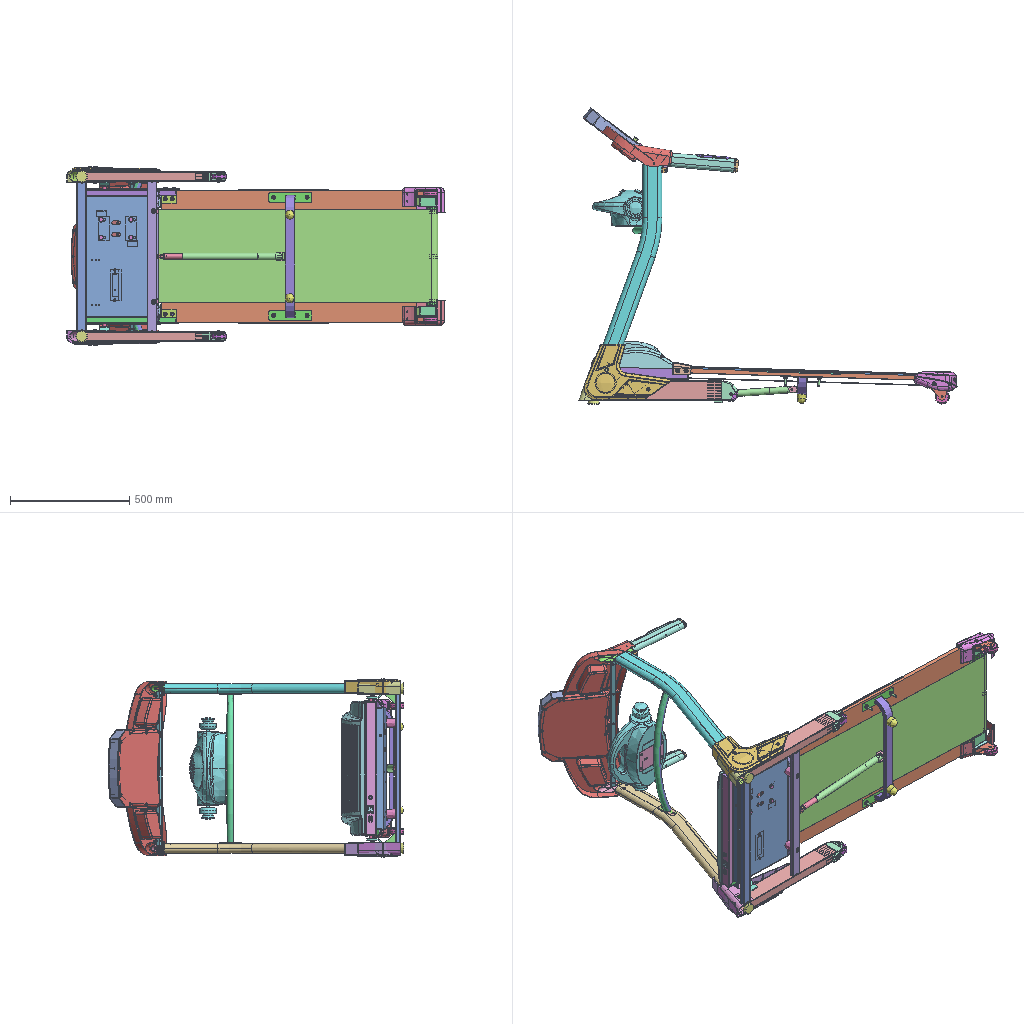Assembly | STEP file | 108 different items | 216 placed | box 1585 x 1241 x 747 mm
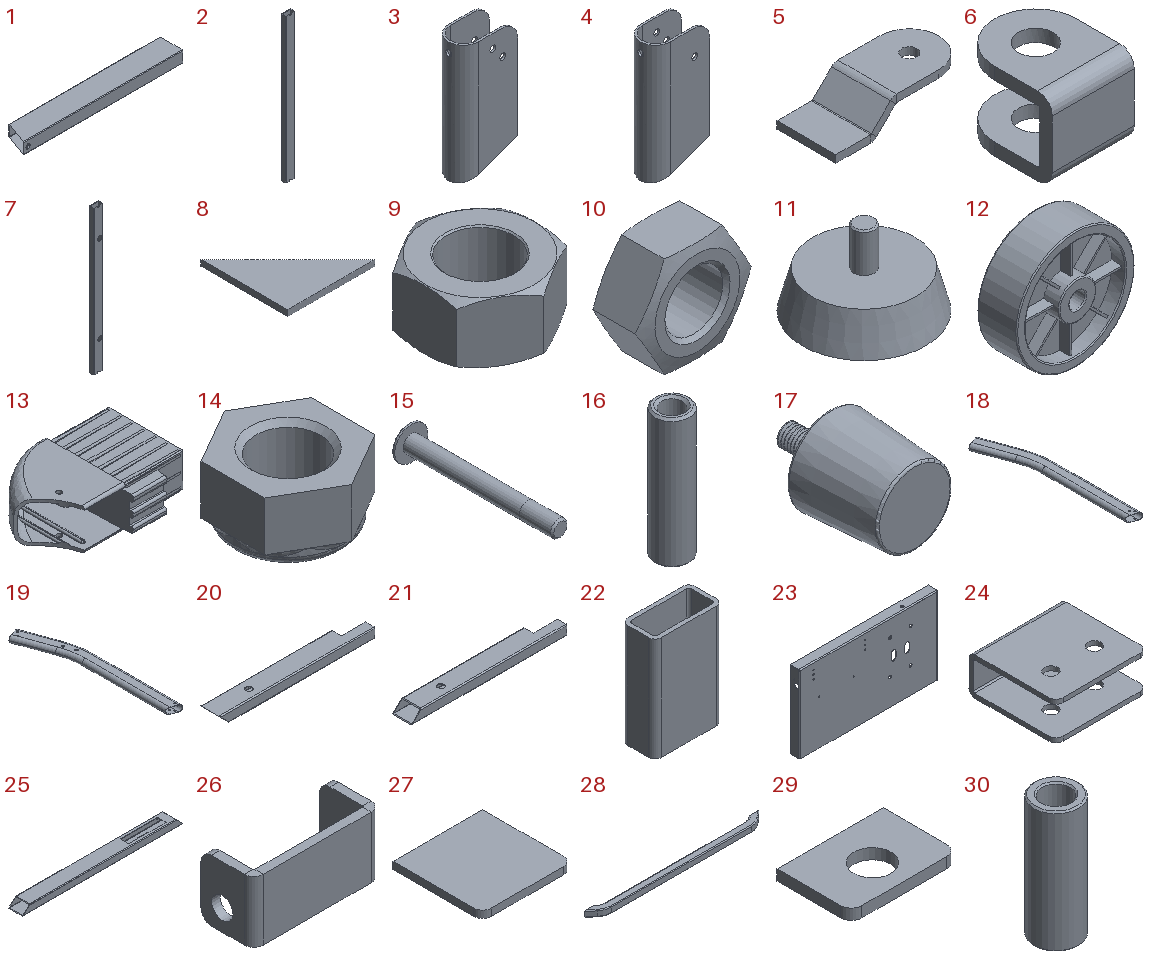Parts list (item | name | quantity | parent item | size | volume):
1 | 5090101 | x2 | in 5090100 | 550 x 80 x 40 mm | 185626 mm3
2 | 5090102 | x1 | in 5090100 | 40 x 20 x 624 mm | 103774 mm3
3 | 5090103L | x1 | in 5090100 | 83 x 46 x 184 mm | 94323 mm3
4 | 5090103R | x1 | in 5090100 | 83 x 46 x 184 mm | 94323 mm3
5 | 5090104 | x2 | in 5090100 | 90 x 40 x 20 mm | 17915 mm3
6 | PN_0010_default | x3 | in 5090100, 5090200L, 5090200R | 20 x 24 x 19 mm | 2959 mm3
7 | 5090107 | x1 | in 5090100 | 40 x 20 x 630 mm | 102888 mm3
8 | 5090108 | x2 | in 5090100 | 45 x 45 x 3 mm | 3037 mm3
9 | N1101210 | x4 | in 5090100, 5091300 | 16.454 x 19 x 9 mm | 1389 mm3
10 | N108078 | x10 | in 5090100, 5090200L, 5090200R, 5091200 | 16 x 7 x 13.856 mm | 779.97 mm3
11 | 5090101W | x2 | in 5090100Z | 47.789 x 47.789 x 30.5 mm | 24412 mm3
12 | PN_0007_default | x2 | in 5090100Z | 60 x 22 x 60 mm | 32782 mm3
13 | PN_0011_default | x2 | in 5090100Z | 130 x 91 x 40 mm | 95148 mm3
14 | PN_0002 | x2 | in 5090100Z | 8.5 x 9.815 x 5.1 mm | 204.852 mm3
15 | SD10545 | x2 | in 5090100Z | 10 x 47.433 x 10 mm | 991.806 mm3
16 | 5090905 | x2 | in 5090100Z | 8.2 x 8.2 x 31 mm | 968.239 mm3
17 | 5090104W | x2 | in 5090100Z | 39.871 x 60 x 39.871 mm | 45524 mm3
18 | 5090201L | x1 | in 5090200L | 181.681 x 917.444 x 40 mm | 273623 mm3
19 | 5090201R | x1 | in 5090200R | 181.681 x 917.444 x 40 mm | 273224 mm3
20 | 5090501L | x1 | in 5090500 | 400 x 50 x 25 mm | 74106 mm3
21 | 5090501R | x1 | in 5090500 | 400 x 50 x 25 mm | 74487 mm3
22 | 5090502 | x2 | in 5090500 | 26 x 13 x 40 mm | 4140 mm3
23 | 5090503 | x1 | in 5090500 | 508 x 35 x 285 mm | 354091 mm3
24 | 5090504 | x4 | in 5090500, 5091400L, 5091400R | 63 x 60 x 26 mm | 24845 mm3
25 | 5090505 | x1 | in 5090500 | 558 x 50 x 25 mm | 105328 mm3
26 | 5090506 | x1 | in 5090500 | 60 x 25 x 29 mm | 10869 mm3
27 | 5090507 | x2 | in 5090500 | 25 x 25 x 2 mm | 1245 mm3
28 | 5090508 | x1 | in 5090500 | 550.086 x 30 x 20 mm | 56532 mm3
29 | 5090509 | x1 | in 5090500 | 50 x 35 x 5 mm | 7494 mm3
30 | 5090510 | x2 | in 5090500 | 15.8 x 15.8 x 43 mm | 5033 mm3
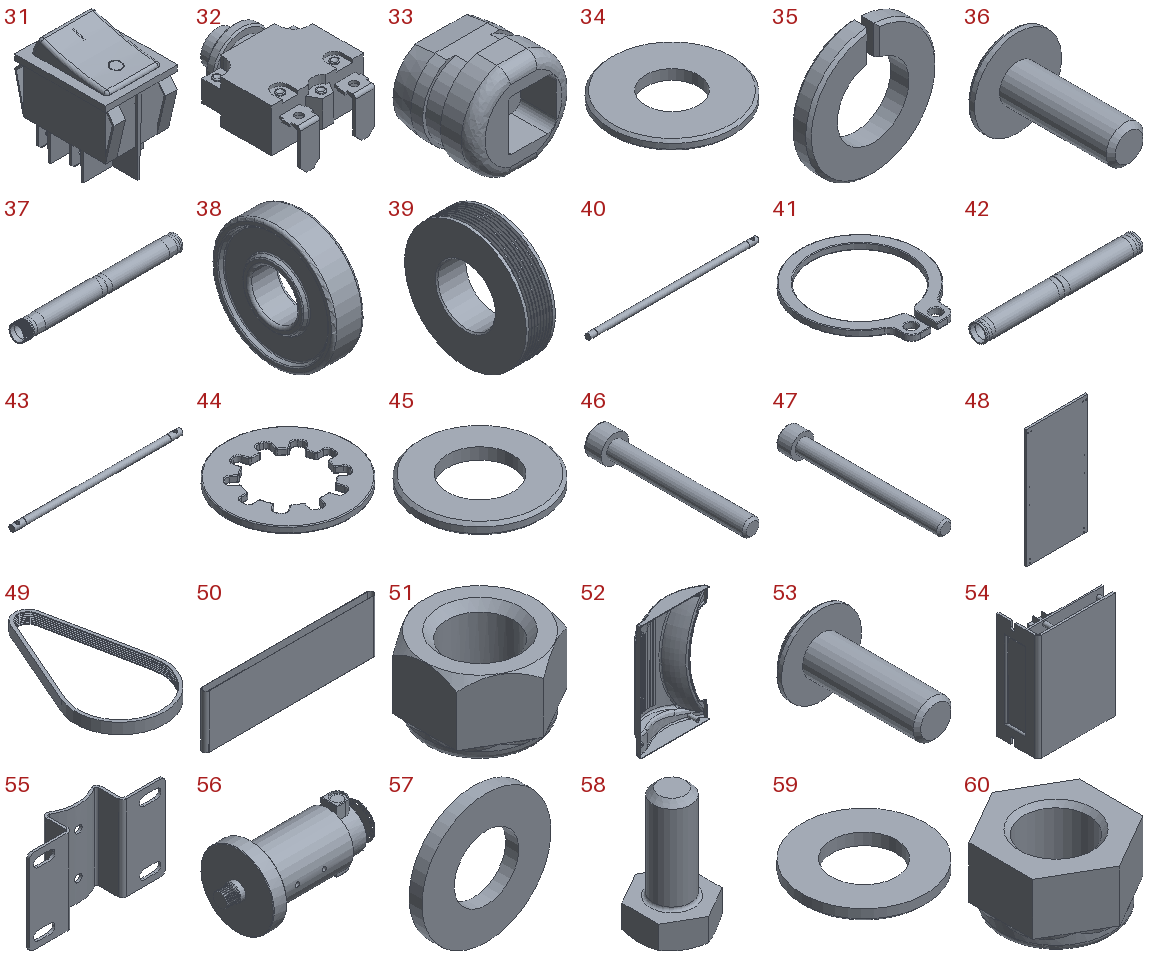31 | EP002 | x1 | in 5090500Z | 25 x 34.5 x 34.784 mm | 14567 mm3
32 | EC002 | x1 | in 5090500Z | 29.3 x 39.3 x 19.65 mm | 10331 mm3
33 | PN_0006_default | x1 | in 5090500Z | 17 x 14 x 16 mm | 1519 mm3
34 | PN_0009 | x3 | in 5090500Z | 9.8 x 9.8 x 0.8 mm | 48.045 mm3
35 | W204009 | x3 | in 5090500Z | 9.2 x 1.3 x 9.193 mm | 57.255 mm3
36 | SD10412 | x3 | in 5090500Z | 9.4 x 14.503 x 9.4 mm | 245.335 mm3
37 | 5090701 | x1 | in 5090700Z | 460 x 46 x 46 mm | 209317 mm3
38 | PL6203ZZA_default | x4 | in 5090700Z, 5090800Z | 11 x 44 x 44 mm | 11669 mm3
39 | PN_0004_default | x1 | in 5090700Z | 23 x 96 x 96 mm | 121730 mm3
40 | 5090702 | x1 | in 5090700Z | 513 x 17 x 17 mm | 116620 mm3
41 | PN_0013 | x4 | in 5090700Z, 5090800Z | 19 x 21.5 x 1 mm | 101.865 mm3
42 | 5090801 | x1 | in 5090800Z | 410 x 46 x 46 mm | 188992 mm3
43 | 5090802 | x1 | in 5090800Z | 480 x 17 x 17 mm | 107509 mm3
44 | PN_0005 | x3 | in 5090500Z | 15 x 15 x 0.8 mm | 82.689 mm3
45 | PN_0008 | x15 | in 5090500Z | 17 x 17 x 1.6 mm | 252.969 mm3
46 | SA10865 | x1 | in 5090500Z | 13 x 73 x 13 mm | 4160 mm3
47 | SA10880 | x2 | in 5090500Z | 13 x 88 x 13 mm | 4914 mm3
48 | DECK509 | x1 | in 5090500Z | 554 x 18 x 1070 mm | 10652247 mm3
49 | DE170J509 | x1 | in 5090500Z | 99 x 178.5 x 12 mm | 14354 mm3
50 | RUBE509 | x1 | in 5090500Z | 1253 x 49.2 x 390 mm | 1595905 mm3
51 | PN_0001 | x2 | in 5090500Z | 10 x 11.547 x 7 mm | 381.046 mm3
52 | MOCV509 | x1 | in 5090500Z | 342.742 x 110.913 x 567 mm | 804281 mm3
53 | SD10515 | x2 | in 5090500Z | 10.5 x 17.955 x 10.5 mm | 436.429 mm3
54 | 509K1002 | x1 | in 5090500Z | 93.5 x 58.5 x 129.5 mm | 128937 mm3
55 | 5090601 | x1 | in 5090500Z | 160 x 33 x 100 mm | 61520 mm3
56 | MOTOR default | x1 | in 5090500Z | 260 x 138 x 138 mm | 1629654 mm3
57 | 509~20.10.T2.0 | x4 | in 5090500Z | 20 x 2 x 20 mm | 471.239 mm3
58 | SI1025_M10 | x4 | in 5090500Z | 17 x 19.6 x 32 mm | 3678 mm3
59 | W110020_M10 | x4 | in 5090500Z | 21 x 21 x 2 mm | 494.539 mm3
60 | N210095 | x4 | in 5090500Z | 17 x 19.63 x 10.5 mm | 1722 mm3
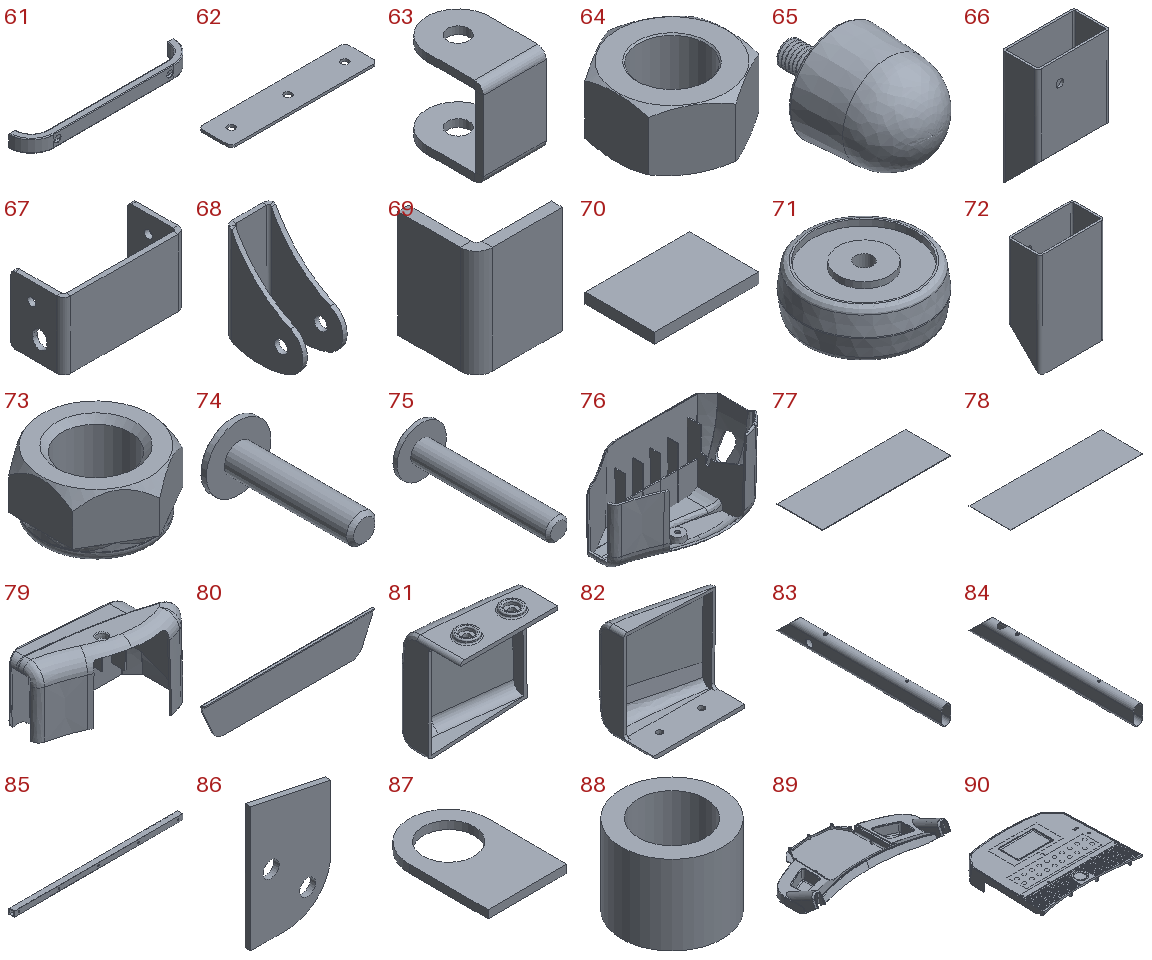61 | 5091301 | x1 | in 5091300 | 515 x 70 x 40 mm | 91933 mm3
62 | 5091302 | x2 | in 5091300 | 180 x 40 x 3 mm | 20963 mm3
63 | 5091303 | x1 | in 5091300 | 25 x 35 x 35 mm | 6553 mm3
64 | N1101215 | x1 | in 5091300 | 16.454 x 19 x 9 mm | 1389 mm3
65 | 5091301W | x2 | in 5091300Z | 39.871 x 60 x 39.871 mm | 39857 mm3
66 | 5091401L | x1 | in 5091400L | 50 x 25 x 80 mm | 14246 mm3
67 | 5091402 | x2 | in 5091400L, 5091400R | 76 x 33 x 42 mm | 16188 mm3
68 | 5091403 | x2 | in 5091400L, 5091400R | 30 x 53 x 70.522 mm | 17329 mm3
69 | 5091404 | x2 | in 5091400L, 5091400R | 24 x 22 x 30 mm | 3754 mm3
70 | 5091405 | x2 | in 5091400L, 5091400R | 30 x 20 x 3 mm | 1800 mm3
71 | Transport wheel | x2 | in 5091400LZ, 5091400RZ | 59.962 x 59.962 x 23 mm | 51034 mm3
72 | 5091401R | x1 | in 5091400R | 50 x 25 x 80 mm | 14246 mm3
73 | N208078 | x12 | in 5090500Z | 13.017 x 15.011 x 7.5 mm | 666.866 mm3
74 | PN_0012 | x6 | in 5090500Z | 18 x 39.451 x 18 mm | 2453 mm3
75 | PN_0003 | x4 | in 5090500Z | 18 x 54.451 x 18 mm | 3207 mm3
76 | END CAP R | x1 | in 5090500Z | 178.531 x 81.742 x 105 mm | 112295 mm3
77 | JZHM | x1 | in 5090500Z | 1060 x 370 x 5 mm | 1961000 mm3
78 | JZBM | x1 | in 5090500Z | 1170 x 370 x 1.5 mm | 649350 mm3
79 | END CAP L | x1 | in 5090500Z | 178.531 x 81.742 x 105 mm | 112297 mm3
80 | Plastic anti-slip plate | x2 | in 5090500Z | 380 x 9.3 x 80 mm | 74474 mm3
81 | HGL | x1 | in 5090500Z | 76.93 x 46.944 x 81.839 mm | 29643 mm3
82 | HGR | x1 | in 5090500Z | 76.93 x 46.944 x 81.839 mm | 29457 mm3
83 | 5091201L | x1 | in 5091200 | 25 x 430 x 50 mm | 72526 mm3
84 | 5091201R | x1 | in 5091200 | 25 x 430 x 50 mm | 72112 mm3
85 | 5091202 | x1 | in 5091200 | 645 x 20 x 20 mm | 70797 mm3
86 | 5091203 | x2 | in 5091200 | 45 x 3 x 70 mm | 8020 mm3
87 | PN_0014_default | x2 | in 5091200 | 20 x 30 x 2 mm | 848.625 mm3
88 | 5091205 | x2 | in 5091200 | 12.7 x 12.7 x 10 mm | 699.319 mm3
89 | 5091204W | x1 | in 5091200ZA | 729.86 x 412.544 x 132.193 mm | 994428 mm3
90 | 5091205W | x1 | in 5091200ZA | 340.656 x 315.859 x 50.2 mm | 442857 mm3
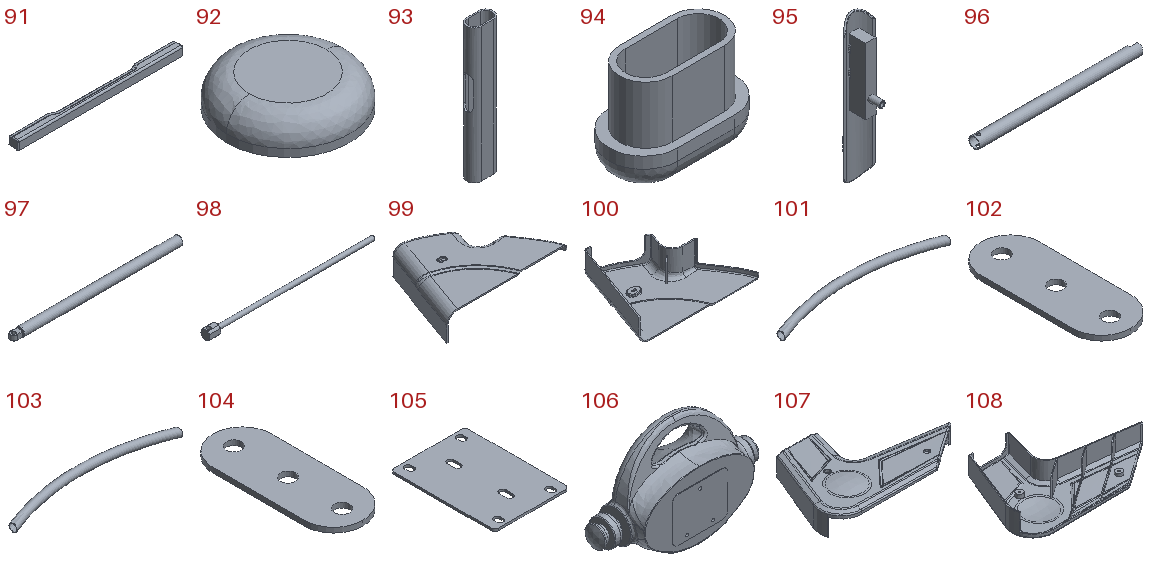91 | 5091206W | x1 | in 5091200ZA | 329.891 x 19 x 17 mm | 29146 mm3
92 | 5091207W | x1 | in 5091200ZA | 32 x 32 x 8 mm | 5722 mm3
93 | 5091202W | x2 | in 5091200Z | 56 x 31 x 280 mm | 111520 mm3
94 | 5091201W | x2 | in 5091200Z | 55 x 30 x 40 mm | 14553 mm3
95 | 5091203W | x2 | in 5091200Z | 31 x 32.516 x 144.3 mm | 20924 mm3
96 | GAS SHOCK A01W | x1 | in 509 | 420 x 28 x 28 mm | 51028 mm3
97 | GAS SHOCK A01X | x1 | in 509 | 419 x 22 x 22 mm | 110141 mm3
98 | GAS SHOCK A01S | x1 | in 509 | 398.5 x 20 x 20 mm | 38228 mm3
99 | LZHT-L1 | x1 | in 509 | 250 x 180.091 x 55 mm | 105552 mm3
100 | LZHT-R1 | x1 | in 509 | 250 x 180.091 x 55 mm | 106562 mm3
101 | 5091501 | x1 | in 5091500 | 620 x 92.341 x 28.6 mm | 81368 mm3
102 | 5091502 | x2 | in 5091500 | 35 x 90 x 3 mm | 8089 mm3
103 | 5091501M | x1 | in 5091500M | 620 x 92.341 x 28.6 mm | 81368 mm3
104 | 5091502M | x2 | in 5091500M | 35 x 90 x 3 mm | 8090 mm3
105 | 5091503M | x1 | in 5091500M | 100 x 140 x 3 mm | 39981 mm3
106 | 5091504W | x1 | in 5091500MA | 430 x 154.443 x 270 mm | 5728271 mm3
107 | BLZHT2-L | x1 | in 509 | 369.553 x 235 x 62.57 mm | 247383 mm3
108 | BLZHT2-R | x1 | in 509 | 369.553 x 235 x 62.57 mm | 247381 mm3
Placements (level | parent | child | x y z in mm | rotation matrix by rows):
1 | 509 | 5090100Z | 20.74 99.795 0.0 | 1 0 0 0 1 0 0 0 1
2 | 5090100Z | 5090100 | -0.0 -0.0 -0.0 | 1 0 0 0 1 0 0 0 1
3 | 5090100 | 5090101 | -0.0 -0.0 -0.0 | 1 0 0 0 1 0 0 0 1
3 | 5090100 | 5090101 | 0.0 -0.0 -670.0 | 1 0 0 0 1 0 0 0 1
3 | 5090100 | 5090102 | -535.0 -0.0 -335.0 | 1 0 0 0 1 0 0 0 1
3 | 5090100 | 5090103L | -526.578 -33.334 0.0 | 0.9397 0 0.342 -0.342 0 0.9397 0 -1 0
3 | 5090100 | 5090103R | -526.578 -33.334 -670.0 | 0.9397 0 0.342 -0.342 0 0.9397 0 -1 -0
3 | 5090100 | 5090104 | -440.0 121.5 -35.0 | 0 1 0 1 0 0 0 0 -1
3 | 5090100 | PN_0010_default | -220.0 10.0 -335.0 | 0 1 0 -1 0 0 0 0 1
3 | 5090100 | 5090104 | -440.0 121.5 -635.0 | 0 -1 0 1 0 0 0 0 1
3 | 5090100 | 5090107 | -240.0 -0.0 -335.0 | 1 0 0 0 1 0 0 0 1
3 | 5090100 | 5090108 | -535.0 28.721 -610.721 | 0 0 1 1 0 0 0 1 -0
3 | 5090100 | N1101210 | -233.0 11.0 -145.0 | 1 0 0 0 0 1 0 -1 0
3 | 5090100 | N1101210 | -233.0 20.0 -525.0 | 1 0 0 0 0 -1 0 1 0
3 | 5090100 | N108078 | -479.683 116.674 -26.5 | 0.7825 0 0.6226 0.6226 0 -0.7825 0 1 -0
3 | 5090100 | N108078 | -479.683 116.674 -643.5 | 0.7825 0 -0.6226 0.6226 0 0.7825 0 -1 -0
3 | 5090100 | 5090108 | -532.0 28.721 -59.279 | 0 0 -1 1 0 0 0 -1 -0
2 | 5090100Z | 5090101W | -535.0 -0.0 -0.0 | 1 0 0 0 0 1 0 -1 0
2 | 5090100Z | PN_0007_default | 40.0 25.0 -11.0 | 1 0 0 0 0 -1 0 1 -0
2 | 5090100Z | PN_0011_default | 70.0 80.0 20.0 | -1 0 0 0 1 0 0 0 -1
2 | 5090100Z | PN_0002 | 40.0 25.0 -23.8 | 1 0 0 0 1 0 0 0 1
2 | 5090100Z | SD10545 | 40.0 25.0 20.0 | 1 0 0 0 0 -1 0 1 0
2 | 5090100Z | 5090905 | 40.0 25.0 15.5 | 1 0 0 0 1 0 0 0 1
2 | 5090100Z | 5090101W | -535.0 -0.0 -670.0 | -1 0 0 0 0 1 0 1 0
2 | 5090100Z | PN_0007_default | 40.0 25.0 -659.0 | -1 0 0 0 0 -1 0 -1 0
2 | 5090100Z | SD10545 | 40.0 25.0 -690.0 | 1 0 0 0 0 1 0 -1 0
2 | 5090100Z | 5090905 | 40.0 25.0 -654.5 | 1 0 0 0 1 0 0 0 1
2 | 5090100Z | PN_0002 | 40.0 25.0 -646.2 | -1 0 0 0 1 0 0 0 -1
2 | 5090100Z | PN_0011_default | 70.0 80.0 -649.992 | -1 0 0 0 1 0 0 0 -1
2 | 5090100Z | 5090104W | -233.0 -8.863 -145.0 | -0.8372 0 -0.5469 0 -1 0 -0.5469 0 0.8372
2 | 5090100Z | 5090104W | -233.0 -8.863 -525.0 | -0.8372 0 0.5469 0 -1 0 0.5469 0 0.8372
1 | 509 | 5090200L | -333.426 643.809 0.0 | 0.9397 0.342 0 -0.342 0.9397 0 0 0 1
2 | 5090200L | 5090201L | -26.789 -424.56 -0.0 | 1 0 0 0 1 0 0 0 1
2 | 5090200L | PN_0010_default | -44.744 430.969 -0.0 | -0.342 0.9397 0 0.9397 0.342 0 0 0 -1
2 | 5090200L | N108078 | 13.211 -426.268 15.0 | 1 0 0 0 0 -1 0 1 0
2 | 5090200L | N108078 | -20.385 -421.442 -0.0 | 0 -1 0 -0.4254 0 -0.905 0.905 0 -0.4254
1 | 509 | 5090200R | -356.082 649.787 -670.0 | 0.9397 0.342 0 -0.342 0.9397 0 0 0 1
2 | 5090200R | 5090201R | -3.454 -422.429 -0.0 | 1 0 0 0 1 0 0 0 1
2 | 5090200R | PN_0010_default | -21.409 433.101 -0.0 | 0.342 0.9397 0 -0.9397 0.342 0 0 0 1
2 | 5090200R | N108078 | 36.546 -424.137 -15.0 | 1 0 0 0 0 -1 0 1 0
2 | 5090200R | N108078 | 2.636 -419.311 -0.0 | 0 -1 0 -0.9664 0 0.2572 -0.2572 0 -0.9664
1 | 509 | 5090500Z | -120.17 187.087 -67.5 | 0.9995 0.03073 0 -0.03073 0.9995 0 0 0 1
2 | 5090500Z | 5090500 | -0.0 -0.0 -0.0 | 1 0 0 0 1 0 0 0 1
3 | 5090500 | 5090501L | -0.0 -0.0 -0.0 | 1 0 0 0 1 0 0 0 1
3 | 5090500 | 5090501R | -0.0 0.0 -535.0 | 1 0 0 0 1 0 0 0 1
3 | 5090500 | 5090502 | -311.0 -21.5 -87.5 | 0 0 1 0 1 0 -1 0 0
3 | 5090500 | 5090502 | -181.0 -21.5 -214.5 | 0 0 -1 0 1 0 1 0 0
3 | 5090500 | 5090503 | -375.0 -30.0 -267.5 | 0 0 -1 0 1 0 1 0 -0
3 | 5090500 | 5090504 | -29.5 37.0 -546.5 | 1 0 0 0 0 1 0 -1 -0
3 | 5090500 | 5090504 | -29.5 37.0 11.5 | 1 0 0 0 0 -1 0 1 -0
3 | 5090500 | 5090505 | -387.5 25.0 -267.5 | 0 0 1 0 1 0 -1 0 -0
3 | 5090500 | 5090506 | -130.0 14.0 -507.0 | -1 0 0 0 1 0 0 0 -1
3 | 5090500 | 5090507 | 2.0 11.5 -0.0 | 0 0 -1 0 1 0 1 0 0
3 | 5090500 | 5090508 | -80.0 -20.0 -267.5 | 0 0 1 0 1 0 -1 0 -0
3 | 5090500 | 5090509 | -130.0 44.0 -17.5 | -1 0 0 0 -1 0 0 0 1
3 | 5090500 | 5090510 | -300.0 25.0 4.0 | 0.9768 -0.2143 0 0.2143 0.9768 0 0 0 1
3 | 5090500 | 5090510 | -300.0 25.0 -539.0 | 0.9768 -0.2143 0 0.2143 0.9768 0 0 0 1
3 | 5090500 | 5090507 | 2.0 11.5 -535.0 | 0 0 -1 0 1 0 1 0 0
2 | 5090500Z | EP002 | -400.0 24.95 -438.75 | 0 0 -1 1 0 0 0 -1 -0
2 | 5090500Z | EC002 | -342.72 18.1 -435.835 | 0 -1 0 0 0 -1 1 0 0
2 | 5090500Z | PN_0006_default | -405.5 24.764 -388.797 | 0 1 0 -1 0 0 0 0 1
2 | 5090500Z | PN_0009 | -255.0 -24.7 -451.5 | 1 0 0 0 0 -1 0 1 -0
2 | 5090500Z | PN_0009 | -254.0 -19.7 -406.5 | -0.9887 -0.15 0 0 0 -1 0.15 -0.9887 -0
2 | 5090500Z | PN_0009 | -255.0 -24.7 -323.5 | 1 0 0 0 0 -1 0 1 -0
2 | 5090500Z | W204009 | -254.0 -19.7 -406.5 | -0.9887 0 -0.15 0 1 0 0.15 0 -0.9887
2 | 5090500Z | W204009 | -255.0 -24.7 -451.5 | 1 0 0 0 1 0 0 0 1
2 | 5090500Z | W204009 | -255.0 -24.7 -323.5 | 1 0 0 0 1 0 0 0 1
2 | 5090500Z | SD10412 | -255.0 -23.4 -323.5 | 0.6736 0 -0.7391 0 1 0 0.7391 0 0.6736
2 | 5090500Z | SD10412 | -254.0 -18.4 -406.5 | 0.923 0 0.3849 0 1 0 -0.3849 0 0.923
2 | 5090500Z | SD10412 | -255.0 -23.4 -451.5 | -0.7187 0 0.6953 0 1 0 -0.6953 0 -0.7187
2 | 5090500Z | 5090700Z | -130.0 29.0 -266.7 | 0 0 1 0 1 0 -1 0 -0
3 | 5090700Z | 5090701 | 0.0 -0.0 0.0 | 1 0 0 0 1 0 0 0 1
3 | 5090700Z | PL6203ZZA_default | -241.0 8.5 -0.0 | 1 0 0 0 1 0 0 0 1
3 | 5090700Z | PL6203ZZA_default | 208.0 8.5 -0.0 | 1 0 0 0 1 0 0 0 1
3 | 5090700Z | PN_0004_default | -218.0 -0.0 0.0 | -1 0 0 0 0.5305 0.8477 0 0.8477 -0.5305
3 | 5090700Z | 5090702 | -7.7 -0.0 0.0 | 1 0 0 0 1 0 0 0 1
3 | 5090700Z | PN_0013 | 220.1 -0.0 0.0 | 0 0 -1 0 1 0 1 0 0
3 | 5090700Z | PN_0013 | -242.1 -0.0 0.0 | 0 0 1 0 1 0 -1 0 0
2 | 5090500Z | 5090800Z | 1074 30.0 -267.0 | 0 0 -1 0 -1 0 -1 0 0
3 | 5090800Z | 5090801 | -0.0 0.0 0.0 | 1 0 0 0 1 0 0 0 1
3 | 5090800Z | 5090802 | -0.0 0.0 0.0 | 1 0 0 0 1 0 0 0 1
3 | 5090800Z | PL6203ZZA_default | -205.0 8.5 -0.0 | 1 0 0 0 1 0 0 0 1
3 | 5090800Z | PL6203ZZA_default | 194.0 8.5 -0.0 | 1 0 0 0 1 0 0 0 1
3 | 5090800Z | PN_0013 | 205.9 0.0 0.0 | 0 0 -1 0 1 0 1 0 0
3 | 5090800Z | PN_0013 | -206.1 0.0 0.0 | 0 0 1 0 1 0 -1 0 -0
2 | 5090500Z | PN_0005 | -160.8 29.0 -502.5 | 0 0 1 -0.6832 -0.7302 0 0.7302 -0.6832 -0
2 | 5090500Z | PN_0005 | 1095.25 30.0 -42.0 | 0 0 1 0.4022 -0.9156 0 0.9156 0.4022 -0
2 | 5090500Z | PN_0005 | 1095.25 30.0 -492.0 | 0 0 1 1 0.003456 0 -0.003456 1 -0
2 | 5090500Z | PN_0008 | -162.4 29.0 -502.5 | 0 0 1 0 1 0 -1 0 0
2 | 5090500Z | PN_0008 | 1097.65 30.0 -492.0 | 0 0 -1 0.4285 -0.9035 0 -0.9035 -0.4285 0
2 | 5090500Z | SA10865 | -162.4 29.0 -502.5 | 0 -1 0 0.4079 0 -0.913 0.913 0 0.4079
2 | 5090500Z | SA10880 | 1097.65 30.0 -42.0 | 0 1 0 -0.354 0 0.9352 0.9352 0 0.354
2 | 5090500Z | SA10880 | 1097.65 30.0 -492.0 | 0 1 0 0.4455 0 0.8953 0.8953 0 -0.4455
2 | 5090500Z | DECK509 | 1010.25 27.0 -267.5 | 0 0 1 0 1 0 -1 0 -0
2 | 5090500Z | DE170J509 | 164.593 508.146 -37.7 | 0.04897 -0.9988 0 0.9988 0.04897 0 0 0 1
2 | 5090500Z | RUBE509 | 1118.5 30.037 -267.5 | 1 -0.000831 0 0.000831 1 0 0 0 1
2 | 5090500Z | PN_0001 | -126.878 5.5 -32.5 | 1 0 0 0 0 1 0 -1 0
2 | 5090500Z | PN_0001 | -126.878 5.5 -502.5 | 1 0 0 0 0 1 0 -1 -0
2 | 5090500Z | MOCV509 | -404.004 41.0 -267.496 | 1 0 0 0 1 0 0 0 1
2 | 5090500Z | SD10515 | 1097.25 35.0 -510.0 | 0 1 0 -0.4667 0 0.8844 0.8844 0 0.4667
2 | 5090500Z | SD10515 | 1097.25 35.0 -25.0 | 0 1 0 0.957 0 -0.29 -0.29 0 -0.957
2 | 5090500Z | 509K1002 | -226.5 -25.5 -453.507 | 0 -1 0 1 0 0 0 0 1
2 | 5090500Z | 5090601 | -243.269 -23.0 -151.0 | 1 0 0 0 1 0 0 0 1
2 | 5090500Z | MOTOR default | -243.269 46.7 -27.5 | 0 0 1 0 1 0 -1 0 -0
2 | 5090500Z | 509~20.10.T2.0 | -186.5 -28.0 -113.5 | 1 0 0 0 1 0 0 0 1
2 | 5090500Z | SI1025_M10 | -186.5 -37.0 -113.5 | 0.9832 -0.1826 0 0 0 1 -0.1826 -0.9832 0
2 | 5090500Z | W110020_M10 | -186.5 -21.0 -113.5 | 1 0 0 0 0 -1 0 1 -0
2 | 5090500Z | N210095 | -186.5 -13.0 -113.5 | 1 0 0 0 0 -1 0 1 -0
2 | 5090500Z | 509~20.10.T2.0 | -311.5 -28.0 -113.5 | 1 0 0 0 1 0 0 0 1
2 | 5090500Z | 509~20.10.T2.0 | -186.5 -28.0 -188.5 | 1 0 0 0 1 0 0 0 1
2 | 5090500Z | 509~20.10.T2.0 | -311.5 -28.0 -188.5 | 1 0 0 0 1 0 0 0 1
2 | 5090500Z | W110020_M10 | -311.5 -21.0 -113.5 | 1 0 0 0 0 -1 0 1 -0
2 | 5090500Z | W110020_M10 | -186.5 -21.0 -188.5 | 1 0 0 0 0 -1 0 1 -0
2 | 5090500Z | W110020_M10 | -311.5 -21.0 -188.5 | 1 0 0 0 0 -1 0 1 -0
2 | 5090500Z | N210095 | -311.5 -13.0 -113.5 | 1 0 0 0 0 -1 0 1 -0
2 | 5090500Z | N210095 | -186.5 -13.0 -188.5 | 1 0 0 0 0 -1 0 1 -0
2 | 5090500Z | N210095 | -311.5 -13.0 -188.5 | 1 0 0 0 0 -1 0 1 -0
2 | 5090500Z | SI1025_M10 | -311.5 -37.0 -113.5 | 0.9832 -0.1826 0 0 0 1 -0.1826 -0.9832 0
2 | 5090500Z | SI1025_M10 | -186.5 -37.0 -188.5 | 0.9832 -0.1826 0 0 0 1 -0.1826 -0.9832 0
2 | 5090500Z | SI1025_M10 | -311.5 -37.0 -188.5 | 0.9832 -0.1826 0 0 0 1 -0.1826 -0.9832 0
2 | 5090500Z | 5091300Z | 480.25 -34.636 -268.287 | 0 0 1 0 1 0 -1 0 0
3 | 5091300Z | 5091300 | 23.777 15.702 0.0 | 1 0 0 0 1 0 0 0 1
4 | 5091300 | 5091301 | -24.565 -17.067 0.0 | 1 0 0 0 1 0 0 0 1
4 | 5091300 | 5091302 | -272.065 45.934 0.0 | 0 -1 0 0 0 -1 1 0 0
4 | 5091300 | 5091302 | 222.935 45.934 0.0 | 0 -1 0 0 0 -1 1 0 0
4 | 5091300 | 5091303 | -24.565 -9.566 -20.0 | 0 0 1 -1 0 0 0 -1 -0
4 | 5091300 | N1101215 | 150.435 -27.067 0.0 | 0.09316 0.9957 0 0 0 1 0.9957 -0.09316 -0
4 | 5091300 | N1101210 | -199.565 -18.067 0.0 | 1 0 0 0 0 -1 0 1 -0
4 | 5091300 | N1101210 | 150.435 -27.067 0.0 | -1 0 0 0 0 1 0 1 0
3 | 5091300Z | 5091301W | -175.787 17.499 0.0 | 1 0 0 0 1 0 0 0 1
3 | 5091300Z | 5091301W | 174.213 17.499 0.0 | 1 0 0 0 1 0 0 0 1
2 | 5090500Z | 5091400LZ | 1025.25 4.175 -18.155 | 0 0 -1 1 0 0 0 -1 0
3 | 5091400LZ | 5091400L | 26.201 -15.308 -30.0 | 1 0 0 0 1 0 0 0 1
4 | 5091400L | 5091401L | -7.375 -1.347 -0.0 | 1 0 0 0 1 0 0 0 1
4 | 5091400L | 5091402 | -15.375 32.153 -40.0 | 0 1 0 0 0 -1 -1 0 0
4 | 5091400L | 5091403 | -32.375 1.153 -1.5 | 0 1 0 -1 0 0 0 0 1
4 | 5091400L | 5091404 | -8.375 1.153 40.0 | 0 -1 0 0 0 -1 1 0 -0
4 | 5091400L | 5090504 | 4.625 17.652 43.0 | 0 0 1 -1 0 0 0 -1 -0
4 | 5091400L | 5091405 | -12.484 34.153 38.883 | 0 0.4109 -0.9117 -1 0 0 0 0.9117 0.4109
3 | 5091400LZ | Transport wheel | -44.175 -25.655 -43.0 | 1 0 0 0 0 1 0 -1 0
2 | 5090500Z | 5091400RZ | 1025.75 -45.789 -505.81 | 0 0 1 -1 0 0 0 -1 -0
3 | 5091400RZ | 5091400R | -65.128 34.772 30.0 | 1 0 0 0 1 0 0 0 1
4 | 5091400R | 5091401R | -3.66 -7.082 -0.5 | -1 0 0 0 1 0 0 0 -1
4 | 5091400R | 5091402 | 4.34 -40.581 -36.5 | 0 -1 0 0 0 1 -1 0 0
4 | 5091400R | 5091403 | 21.34 -9.582 1.0 | 0 -1 0 -1 0 0 0 0 -1
4 | 5091400R | 5091404 | -2.66 -9.582 -40.5 | 0 1 0 0 0 -1 -1 0 -0
4 | 5091400R | 5090504 | -15.66 -26.081 -43.5 | 0 0 -1 -1 0 0 0 1 -0
4 | 5091400R | 5091405 | 4.183 -42.581 -40.616 | 0 -0.4109 -0.9117 1 0 0 0 -0.9117 0.4109
3 | 5091400RZ | Transport wheel | -5.789 13.69 42.5 | 0.9998 -0.02049 0 0 0 1 -0.02049 -0.9998 -0
2 | 5090500Z | PN_0008 | 1097.65 30.0 -42.0 | 0 0 -1 -0.7284 -0.6851 0 -0.6851 0.7284 0
2 | 5090500Z | N208078 | 975.25 14.9 -5.5 | 0.2304 -0.9731 0 0 0 1 -0.9731 -0.2304 0
2 | 5090500Z | PN_0012 | 975.25 48.0 -5.5 | 0.8264 0 -0.563 0 1 0 0.563 0 0.8264
2 | 5090500Z | PN_0003 | 550.25 38.0 -20.0 | 1 0 0 0 1 0 0 0 1
2 | 5090500Z | PN_0008 | 975.25 22.0 -5.5 | 0.1888 -0.982 0 0 0 -1 0.982 0.1888 0
2 | 5090500Z | PN_0012 | 975.25 48.0 -35.5 | 1 0 0 0 1 0 0 0 1
2 | 5090500Z | N208078 | 975.25 14.9 -35.5 | 0.2304 -0.9731 0 0 0 1 -0.9731 -0.2304 0
2 | 5090500Z | PN_0008 | 975.25 22.0 -35.5 | 0.9849 0.1729 0 0 0 -1 -0.1729 0.9849 0
2 | 5090500Z | PN_0012 | -44.5 50.0 -25.5 | 0.8286 0 -0.5599 0 1 0 0.5599 0 0.8286
2 | 5090500Z | N208078 | -44.5 16.9 -25.5 | 0.2318 -0.9728 0 0 0 1 -0.9728 -0.2318 0
2 | 5090500Z | PN_0008 | -44.5 24.0 -25.5 | 0.1877 -0.9822 0 0 0 -1 0.9822 0.1877 0
2 | 5090500Z | PN_0008 | -14.5 24.0 -25.5 | 0.1877 -0.9822 0 0 0 -1 0.9822 0.1877 0
2 | 5090500Z | N208078 | -14.5 16.9 -25.5 | 0.2318 -0.9728 0 0 0 1 -0.9728 -0.2318 0
2 | 5090500Z | PN_0012 | -14.5 50.0 -25.5 | 0.8286 0 -0.5599 0 1 0 0.5599 0 0.8286
2 | 5090500Z | END CAP R | 950.25 64.6 -503.5 | 1 0 0 0 1 0 0 0 1
2 | 5090500Z | PN_0008 | 975.25 22.0 -529.5 | 0.9849 0.1729 0 0 0 -1 -0.1729 0.9849 0
2 | 5090500Z | N208078 | 975.25 14.9 -529.5 | 0.2304 -0.9731 0 0 0 1 -0.9731 -0.2304 0
2 | 5090500Z | PN_0008 | 975.25 22.0 -499.5 | 0.1888 -0.982 0 0 0 -1 0.982 0.1888 0
2 | 5090500Z | N208078 | 975.25 14.9 -499.5 | 0.2304 -0.9731 0 0 0 1 -0.9731 -0.2304 0
2 | 5090500Z | PN_0012 | 975.25 48.0 -499.5 | 0.8264 0 -0.563 0 1 0 0.563 0 0.8264
2 | 5090500Z | PN_0012 | 975.25 48.0 -529.5 | 1 0 0 0 1 0 0 0 1
2 | 5090500Z | N208078 | 550.25 16.9 -20.0 | 0.7312 -0.6821 0 0 0 1 -0.6821 -0.7312 0
2 | 5090500Z | PN_0008 | 550.25 24.0 -20.0 | -0.654 -0.7565 0 0 0 -1 0.7565 -0.654 0
2 | 5090500Z | PN_0003 | 550.25 38.0 -515.0 | 1 0 0 0 1 0 0 0 1
2 | 5090500Z | PN_0008 | 550.25 24.0 -515.0 | -0.654 -0.7565 0 0 0 -1 0.7565 -0.654 0
2 | 5090500Z | N208078 | 550.25 16.9 -515.0 | 0.7312 -0.6821 0 0 0 1 -0.6821 -0.7312 0
2 | 5090500Z | N208078 | 410.25 16.9 -20.0 | 0.2304 -0.9731 0 0 0 1 -0.9731 -0.2304 -0
2 | 5090500Z | PN_0003 | 410.25 38.0 -20.0 | 0.5998 0 0.8001 0 1 0 -0.8001 0 0.5998
2 | 5090500Z | PN_0008 | 410.25 24.0 -20.0 | -0.8784 -0.478 0 0 0 -1 0.478 -0.8784 0
2 | 5090500Z | PN_0003 | 410.25 38.0 -515.0 | 0.5998 0 -0.8001 0 1 0 0.8001 0 0.5998
2 | 5090500Z | N208078 | 410.25 16.9 -515.0 | -0.2304 -0.9731 0 0 0 1 -0.9731 0.2304 0
2 | 5090500Z | PN_0008 | 410.25 22.4 -515.0 | -0.8784 -0.478 0 0 0 1 -0.478 0.8784 0
2 | 5090500Z | JZHM | 425.25 50.0 -267.5 | 1 0 0 0 0 -1 0 1 0
2 | 5090500Z | JZBM | 425.25 50.0 -267.5 | 1 0 0 0 0 1 0 -1 -0
2 | 5090500Z | END CAP L | 950.25 64.6 -31.5 | 1 0 0 0 1 0 0 0 1
2 | 5090500Z | N208078 | -44.5 16.9 -509.5 | -0.2318 -0.9728 0 0 0 1 -0.9728 0.2318 -0
2 | 5090500Z | N208078 | -14.5 16.9 -509.5 | -0.2318 -0.9728 0 0 0 1 -0.9728 0.2318 -0
2 | 5090500Z | PN_0008 | -14.5 22.4 -509.5 | 0.1877 -0.9822 0 0 0 1 -0.9822 -0.1877 0
2 | 5090500Z | PN_0008 | -44.5 22.4 -509.5 | 0.1877 -0.9822 0 0 0 1 -0.9822 -0.1877 0
2 | 5090500Z | Plastic anti-slip plate | 351.632 40.6 -47.456 | 1 0 0 0 1 0 0 0 1
2 | 5090500Z | Plastic anti-slip plate | 548.306 40.6 -487.544 | -1 0 0 0 1 0 0 0 -1
2 | 5090500Z | HGL | -24.504 34.164 -22.0 | 1 0 0 0 1 0 0 0 1
2 | 5090500Z | HGR | -25.5 38.0 -508.0 | 1 0 0 0 1 0 0 0 1
1 | 509 | 5091200Z | 75.762 1083.904 0.0 | 0 -0.9962 -0.08716 0 0.08716 -0.9962 1 0 -0
2 | 5091200Z | 5091200 | -0.0 -0.0 -0.0 | 1 0 0 0 1 0 0 0 1
3 | 5091200 | 5091201L | -0.0 -0.0 -0.0 | 1 0 0 0 1 0 0 0 1
3 | 5091200 | 5091201R | -670.0 0.0 -0.0 | 1 0 0 0 1 0 0 0 1
3 | 5091200 | 5091202 | -335.0 373.78 5.28 | 1 0 0 0 -0.5299 0.848 0 -0.848 -0.5299
3 | 5091200 | 5091203 | -14.0 341.552 39.935 | 0 1 0 0.9781 0 -0.2079 -0.2079 0 -0.9781
3 | 5091200 | PN_0014_default | -0.0 287.0 24.998 | 0 0 -1 -1 0.000175 0 0.000175 1 -0
3 | 5091200 | 5091205 | -0.0 287.003 44.998 | 0 0 1 0 1 0 -1 0 0
3 | 5091200 | 5091203 | -656.0 341.552 39.935 | 0 1 0 0.9781 0 -0.2079 -0.2079 0 -0.9781
3 | 5091200 | PN_0014_default | -670.0 287.0 24.998 | 0 0 -1 -1 0.000175 0 0.000175 1 -0
3 | 5091200 | N108078 | -9.0 331.0 43.2 | 0 1 0 -0.8676 0 0.4973 0.4973 0 0.8676
3 | 5091200 | N108078 | -661.0 331.0 43.2 | 0 -1 0 -0.8676 0 -0.4973 0.4973 0 -0.8676
3 | 5091200 | 5091205 | -670.0 287.003 44.998 | 0 0 1 0 1 0 -1 0 0
3 | 5091200 | N108078 | -9.0 355.002 57.523 | 0 1 0 -0.8676 0 0.4973 0.4973 0 0.8676
3 | 5091200 | N108078 | -661.0 355.002 57.523 | 0 -1 0 -0.8676 0 -0.4973 0.4973 0 -0.8676
2 | 5091200Z | 5091200ZA | -365.085 410.149 -48.402 | -1 0 0 0 0.848 -0.5299 0 -0.5299 -0.848
3 | 5091200ZA | 5091204W | -30.085 73.92 -34.345 | 1 0 0 0 1 0 0 0 1
3 | 5091200ZA | 5091205W | -30.085 73.92 -31.145 | 1 0 0 0 1 0 0 0 1
3 | 5091200ZA | 5091206W | -30.085 73.92 -31.345 | 1 0 0 0 1 0 0 0 1
3 | 5091200ZA | 5091207W | -30.085 73.92 -31.145 | 1 0 0 0 1 0 0 0 1
2 | 5091200Z | 5091202W | -0.0 279.807 -0.0 | 0 -1 0 0 0 -1 1 0 0
2 | 5091200Z | 5091202W | -670.0 280.0 0.0 | 0 -1 0 0 0 -1 1 0 0
2 | 5091200Z | 5091201W | -0.0 -15.0 0.0 | 0 -1 0 0 0 1 -1 0 -0
2 | 5091200Z | 5091201W | -670.0 -15.0 0.0 | 0 1 0 0 0 1 1 0 -0
2 | 5091200Z | 5091203W | 0.0 18.803 -12.5 | 1 0 0 0 0 1 0 -1 -0
2 | 5091200Z | 5091203W | -670.0 18.803 -12.5 | 1 0 0 0 0 1 0 -1 -0
1 | 509 | GAS SHOCK A01W | 326.473 145.85 -335.0 | -0.9975 -0.07028 0 -0.07028 0.9975 0 0 0 -1
1 | 509 | GAS SHOCK A01X | 9.757 123.535 -335.0 | 0.9975 -0.07028 0 0.07028 0.9975 0 0 0 1
1 | 509 | GAS SHOCK A01S | 296.547 143.742 -335.0 | -0.9975 0.07028 0 -0.07028 -0.9975 0 0 0 1
1 | 509 | LZHT-L1 | -543.852 191.542 -29.0 | 1 0 0 0 1 0 0 0 1
1 | 509 | LZHT-R1 | -543.852 191.542 -641.0 | 1 0 0 0 1 0 0 0 1
1 | 509 | 5091500 | -313.837 812.018 -32.373 | 0 -1 0.003784 0 0.003784 1 -1 0 -0
2 | 5091500 | 5091501 | 302.627 -55.559 0.0 | 1 0 0 0 1 0 0 0 1
2 | 5091500 | 5091502 | -7.373 -40.559 -0.5 | 0 0 -1 -1 0 0 0 1 -0
2 | 5091500 | 5091502 | 615.626 -40.559 -0.5 | 0 0 -1 -1 0 0 0 1 0
1 | 509 | 5091500MA | -313.337 812.016 -32.373 | 0 -1 0.003784 0 0.003784 1 -1 0 0
2 | 5091500MA | 5091500M | -0.0 -0.0 -0.0 | 1 0 0 0 1 0 0 0 1
3 | 5091500M | 5091501M | 302.627 -55.559 0.0 | 1 0 0 0 1 0 0 0 1
3 | 5091500M | 5091502M | -7.373 -40.059 -0.5 | 0 0 -1 -1 0 0 0 1 0
3 | 5091500M | 5091502M | 615.626 -40.059 -0.5 | 0 0 -1 -1 0 0 0 1 0
3 | 5091500M | 5091503M | 302.627 39.441 14.3 | -1 0 0 0 -1 0 0 0 1
2 | 5091500MA | 5091504W | 302.627 55.441 18.8 | -1 0 0 0 0 1 0 1 -0
1 | 509 | BLZHT2-L | -179.869 186.309 4.824 | 1 0 0 0 1 0 0 0 1
1 | 509 | BLZHT2-R | -179.869 186.309 -671.0 | 1 0 0 0 1 0 0 0 1